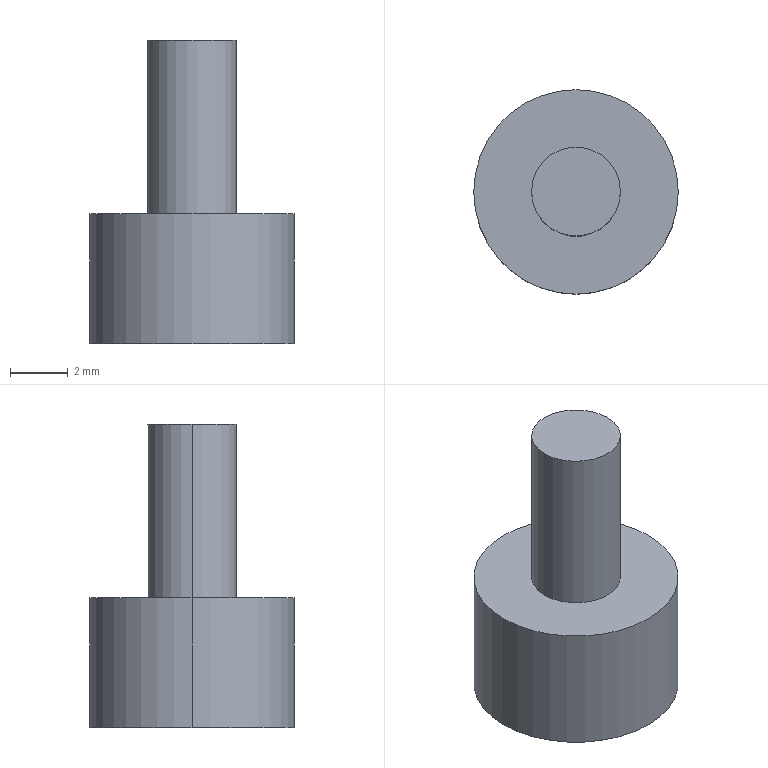Part | SolidWorks | features Extrusion 1, ICE 1 | 1 solid | 7 faces | box 7.08 x 7.08 x 10.5 mm | volume 221.865 mm3 | cylinder 4 | plane 3 | commonest cylinder face diameters 3.08 x2 7.08 x2
STEP:
#1=CARTESIAN_POINT('',(1.54,0.,10.5));
#2=VERTEX_POINT('',#1);
#3=CARTESIAN_POINT('',(-1.54,0.,10.5));
#4=VERTEX_POINT('',#3);
#5=CARTESIAN_POINT('',(0.,0.,10.5));
#6=DIRECTION('',(0.,0.,1.));
#7=DIRECTION('',(1.,0.,0.));
#8=AXIS2_PLACEMENT_3D('',#5,#6,#7);
#9=CIRCLE('',#8,1.54);
#10=EDGE_CURVE('',#2,#4,#9,.T.);
#11=ORIENTED_EDGE('',*,*,#10,.F.);
#12=CARTESIAN_POINT('',(1.54,0.,4.5));
#13=VERTEX_POINT('',#12);
#14=CARTESIAN_POINT('',(1.54,0.,10.5));
#15=DIRECTION('',(0.,0.,-1.));
#16=VECTOR('',#15,1000.);
#17=LINE('',#14,#16);
#18=EDGE_CURVE('',#2,#13,#17,.T.);
#19=ORIENTED_EDGE('',*,*,#18,.T.);
#20=CARTESIAN_POINT('',(-1.54,0.,4.5));
#21=VERTEX_POINT('',#20);
#22=CARTESIAN_POINT('',(0.,0.,4.5));
#23=DIRECTION('',(0.,0.,1.));
#24=DIRECTION('',(1.,0.,0.));
#25=AXIS2_PLACEMENT_3D('',#22,#23,#24);
#26=CIRCLE('',#25,1.54);
#27=EDGE_CURVE('',#13,#21,#26,.T.);
#28=ORIENTED_EDGE('',*,*,#27,.T.);
#29=CARTESIAN_POINT('',(-1.54,0.,10.5));
#30=DIRECTION('',(0.,0.,-1.));
#31=VECTOR('',#30,1000.);
#32=LINE('',#29,#31);
#33=EDGE_CURVE('',#4,#21,#32,.T.);
#34=ORIENTED_EDGE('',*,*,#33,.F.);
#35=EDGE_LOOP('',(#11,#19,#28,#34));
#36=FACE_OUTER_BOUND('',#35,.T.);
#37=CARTESIAN_POINT('',(0.,0.,10.5));
#38=DIRECTION('',(0.,0.,-1.));
#39=DIRECTION('',(-1.,0.,0.));
#40=AXIS2_PLACEMENT_3D('',#37,#38,#39);
#41=CYLINDRICAL_SURFACE('',#40,1.54);
#42=ADVANCED_FACE('',(#36),#41,.T.);
#43=CARTESIAN_POINT('',(3.54,0.,4.5));
#44=VERTEX_POINT('',#43);
#45=CARTESIAN_POINT('',(-3.54,0.,4.5));
#46=VERTEX_POINT('',#45);
#47=CARTESIAN_POINT('',(0.,0.,4.5));
#48=DIRECTION('',(0.,0.,1.));
#49=DIRECTION('',(1.,0.,0.));
#50=AXIS2_PLACEMENT_3D('',#47,#48,#49);
#51=CIRCLE('',#50,3.54);
#52=EDGE_CURVE('',#44,#46,#51,.T.);
#53=ORIENTED_EDGE('',*,*,#52,.F.);
#54=CARTESIAN_POINT('',(3.54,0.,0.));
#55=VERTEX_POINT('',#54);
#56=CARTESIAN_POINT('',(3.54,0.,4.5));
#57=DIRECTION('',(0.,0.,-1.));
#58=VECTOR('',#57,1000.);
#59=LINE('',#56,#58);
#60=EDGE_CURVE('',#44,#55,#59,.T.);
#61=ORIENTED_EDGE('',*,*,#60,.T.);
#62=CARTESIAN_POINT('',(-3.54,0.,0.));
#63=VERTEX_POINT('',#62);
#64=CARTESIAN_POINT('',(0.,0.,0.));
#65=DIRECTION('',(0.,0.,1.));
#66=DIRECTION('',(1.,0.,0.));
#67=AXIS2_PLACEMENT_3D('',#64,#65,#66);
#68=CIRCLE('',#67,3.54);
#69=EDGE_CURVE('',#55,#63,#68,.T.);
#70=ORIENTED_EDGE('',*,*,#69,.T.);
#71=CARTESIAN_POINT('',(-3.54,0.,4.5));
#72=DIRECTION('',(0.,0.,-1.));
#73=VECTOR('',#72,1000.);
#74=LINE('',#71,#73);
#75=EDGE_CURVE('',#46,#63,#74,.T.);
#76=ORIENTED_EDGE('',*,*,#75,.F.);
#77=EDGE_LOOP('',(#53,#61,#70,#76));
#78=FACE_OUTER_BOUND('',#77,.T.);
#79=CARTESIAN_POINT('',(0.,0.,4.5));
#80=DIRECTION('',(0.,0.,-1.));
#81=DIRECTION('',(-1.,0.,0.));
#82=AXIS2_PLACEMENT_3D('',#79,#80,#81);
#83=CYLINDRICAL_SURFACE('',#82,3.54);
#84=ADVANCED_FACE('',(#78),#83,.T.);
#85=ORIENTED_EDGE('',*,*,#60,.F.);
#86=CARTESIAN_POINT('',(0.,0.,4.5));
#87=DIRECTION('',(0.,0.,1.));
#88=DIRECTION('',(1.,0.,0.));
#89=AXIS2_PLACEMENT_3D('',#86,#87,#88);
#90=CIRCLE('',#89,3.54);
#91=EDGE_CURVE('',#46,#44,#90,.T.);
#92=ORIENTED_EDGE('',*,*,#91,.F.);
#93=ORIENTED_EDGE('',*,*,#75,.T.);
#94=CARTESIAN_POINT('',(0.,0.,0.));
#95=DIRECTION('',(0.,0.,1.));
#96=DIRECTION('',(1.,0.,0.));
#97=AXIS2_PLACEMENT_3D('',#94,#95,#96);
#98=CIRCLE('',#97,3.54);
#99=EDGE_CURVE('',#63,#55,#98,.T.);
#100=ORIENTED_EDGE('',*,*,#99,.T.);
#101=EDGE_LOOP('',(#85,#92,#93,#100));
#102=FACE_OUTER_BOUND('',#101,.T.);
#103=CARTESIAN_POINT('',(0.,0.,4.5));
#104=DIRECTION('',(0.,0.,-1.));
#105=DIRECTION('',(-1.,0.,0.));
#106=AXIS2_PLACEMENT_3D('',#103,#104,#105);
#107=CYLINDRICAL_SURFACE('',#106,3.54);
#108=ADVANCED_FACE('',(#102),#107,.T.);
#109=CARTESIAN_POINT('',(0.,0.,4.5));
#110=DIRECTION('',(0.,0.,1.));
#111=DIRECTION('',(1.,0.,0.));
#112=AXIS2_PLACEMENT_3D('',#109,#110,#111);
#113=CIRCLE('',#112,1.54);
#114=EDGE_CURVE('',#21,#13,#113,.T.);
#115=ORIENTED_EDGE('',*,*,#114,.F.);
#116=ORIENTED_EDGE('',*,*,#27,.F.);
#117=EDGE_LOOP('',(#115,#116));
#118=FACE_BOUND('',#117,.T.);
#119=ORIENTED_EDGE('',*,*,#91,.T.);
#120=ORIENTED_EDGE('',*,*,#52,.T.);
#121=EDGE_LOOP('',(#119,#120));
#122=FACE_OUTER_BOUND('',#121,.T.);
#123=CARTESIAN_POINT('',(0.,0.,4.5));
#124=DIRECTION('',(0.,0.,1.));
#125=DIRECTION('',(1.,0.,0.));
#126=AXIS2_PLACEMENT_3D('',#123,#124,#125);
#127=PLANE('',#126);
#128=ADVANCED_FACE('',(#118,#122),#127,.T.);
#129=ORIENTED_EDGE('',*,*,#99,.F.);
#130=ORIENTED_EDGE('',*,*,#69,.F.);
#131=EDGE_LOOP('',(#129,#130));
#132=FACE_OUTER_BOUND('',#131,.T.);
#133=CARTESIAN_POINT('',(0.,0.,0.));
#134=DIRECTION('',(0.,0.,1.));
#135=DIRECTION('',(1.,0.,0.));
#136=AXIS2_PLACEMENT_3D('',#133,#134,#135);
#137=PLANE('',#136);
#138=ADVANCED_FACE('',(#132),#137,.F.);
#139=ORIENTED_EDGE('',*,*,#18,.F.);
#140=CARTESIAN_POINT('',(0.,0.,10.5));
#141=DIRECTION('',(0.,0.,1.));
#142=DIRECTION('',(1.,0.,0.));
#143=AXIS2_PLACEMENT_3D('',#140,#141,#142);
#144=CIRCLE('',#143,1.54);
#145=EDGE_CURVE('',#4,#2,#144,.T.);
#146=ORIENTED_EDGE('',*,*,#145,.F.);
#147=ORIENTED_EDGE('',*,*,#33,.T.);
#148=ORIENTED_EDGE('',*,*,#114,.T.);
#149=EDGE_LOOP('',(#139,#146,#147,#148));
#150=FACE_OUTER_BOUND('',#149,.T.);
#151=CARTESIAN_POINT('',(0.,0.,10.5));
#152=DIRECTION('',(0.,0.,-1.));
#153=DIRECTION('',(-1.,0.,0.));
#154=AXIS2_PLACEMENT_3D('',#151,#152,#153);
#155=CYLINDRICAL_SURFACE('',#154,1.54);
#156=ADVANCED_FACE('',(#150),#155,.T.);
#157=ORIENTED_EDGE('',*,*,#145,.T.);
#158=ORIENTED_EDGE('',*,*,#10,.T.);
#159=EDGE_LOOP('',(#157,#158));
#160=FACE_OUTER_BOUND('',#159,.T.);
#161=CARTESIAN_POINT('',(0.,0.,10.5));
#162=DIRECTION('',(0.,0.,1.));
#163=DIRECTION('',(1.,0.,0.));
#164=AXIS2_PLACEMENT_3D('',#161,#162,#163);
#165=PLANE('',#164);
#166=ADVANCED_FACE('',(#160),#165,.T.);
#167=CLOSED_SHELL('',(#42,#84,#108,#128,#138,#156,#166));
#168=MANIFOLD_SOLID_BREP('',#167);
#169=CARTESIAN_POINT('',(0.,0.,0.));
#170=DIRECTION('',(0.,0.,1.));
#171=DIRECTION('',(1.,0.,0.));
#172=AXIS2_PLACEMENT_3D('',#169,#170,#171);
#173=(LENGTH_UNIT()NAMED_UNIT(*)SI_UNIT(.MILLI.,.METRE.));
#174=UNCERTAINTY_MEASURE_WITH_UNIT(LENGTH_MEASURE(0.00001),#173,'','');
#175=(NAMED_UNIT(*)PLANE_ANGLE_UNIT()SI_UNIT($,.RADIAN.));
#176=(NAMED_UNIT(*)SI_UNIT($,.STERADIAN.)SOLID_ANGLE_UNIT());
#177=(GEOMETRIC_REPRESENTATION_CONTEXT(3)GLOBAL_UNCERTAINTY_ASSIGNED_CONTEXT((#174))GLOBAL_UNIT_ASSIGNED_CONTEXT((#173,#175,#176))REPRESENTATION_CONTEXT('',''));
#178=ADVANCED_BREP_SHAPE_REPRESENTATION('',(#168,#172),#177);